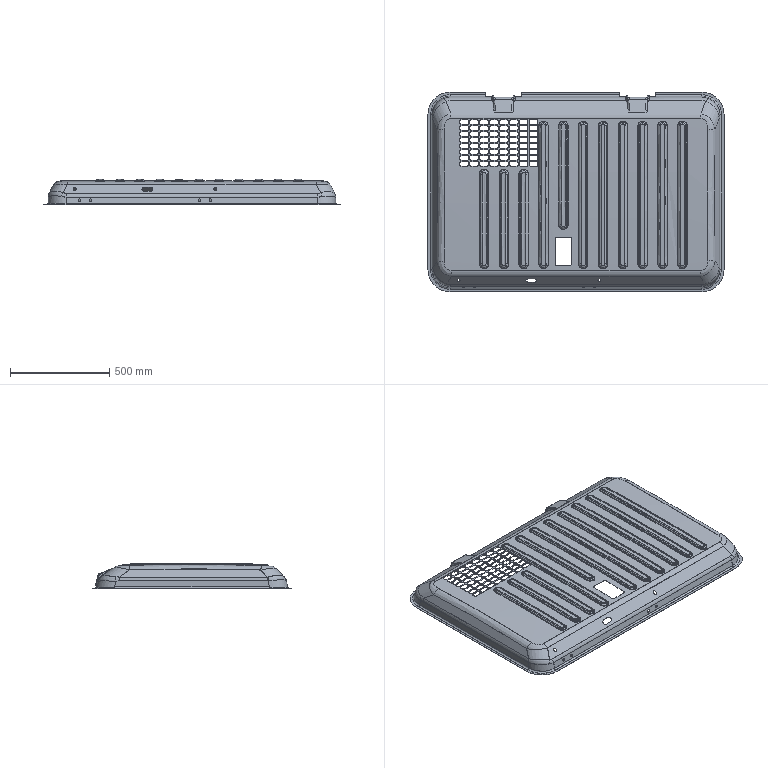Part | SolidWorks | features MBimport 1 | 1 solid | 1196 faces | box 1493 x 1007 x 129.32 mm | volume 2089478 mm3 | spline 764 | plane 326 | cylinder 106 | commonest cylinder face diameters 24014 x11 24016 x11 12.5 x8 77.6 x8 80 x8 177.6 x8